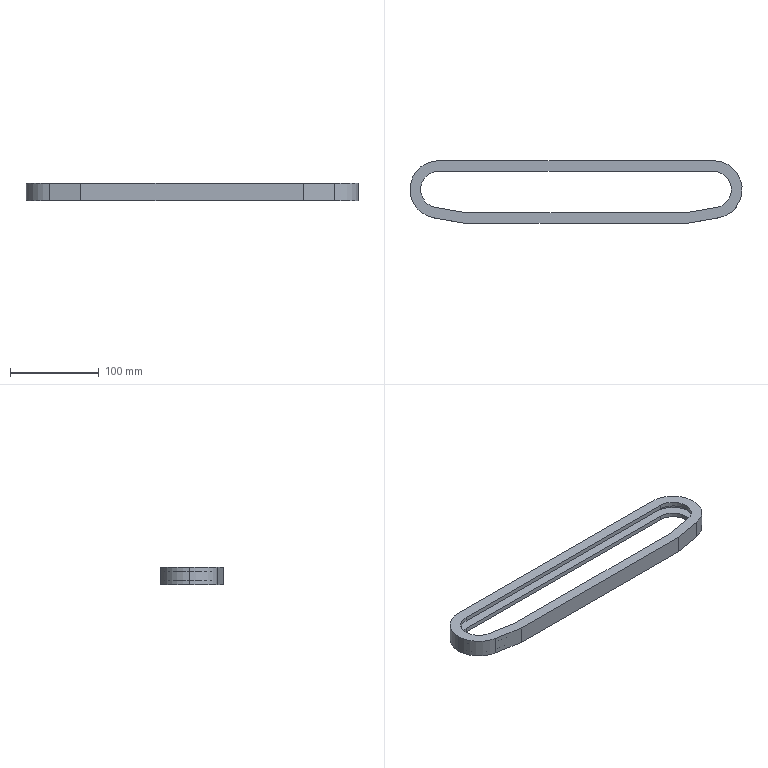Part | SolidWorks | features Extrusion 1, ICE 1 | 1 solid | 32 faces | box 375 x 70.699 x 20 mm | volume 102724 mm3 | plane 20 | cylinder 12 | commonest cylinder face diameters 41 x6 63 x3 65 x3
STEP:
#1=CARTESIAN_POINT('',(186.5,0.,-5.));
#2=VERTEX_POINT('',#1);
#3=CARTESIAN_POINT('',(155.,31.5,-5.));
#4=VERTEX_POINT('',#3);
#5=CARTESIAN_POINT('',(155.,0.,-5.));
#6=DIRECTION('',(0.,0.,1.));
#7=DIRECTION('',(1.,0.,0.));
#8=AXIS2_PLACEMENT_3D('',#5,#6,#7);
#9=CIRCLE('',#8,31.5);
#10=EDGE_CURVE('',#2,#4,#9,.T.);
#11=ORIENTED_EDGE('',*,*,#10,.F.);
#12=CARTESIAN_POINT('',(186.5,0.,5.));
#13=VERTEX_POINT('',#12);
#14=CARTESIAN_POINT('',(186.5,0.,-5.));
#15=DIRECTION('',(0.,0.,1.));
#16=VECTOR('',#15,1000.);
#17=LINE('',#14,#16);
#18=EDGE_CURVE('',#2,#13,#17,.T.);
#19=ORIENTED_EDGE('',*,*,#18,.T.);
#20=CARTESIAN_POINT('',(155.,31.5,5.));
#21=VERTEX_POINT('',#20);
#22=CARTESIAN_POINT('',(155.,0.,5.));
#23=DIRECTION('',(0.,0.,1.));
#24=DIRECTION('',(1.,0.,0.));
#25=AXIS2_PLACEMENT_3D('',#22,#23,#24);
#26=CIRCLE('',#25,31.5);
#27=EDGE_CURVE('',#13,#21,#26,.T.);
#28=ORIENTED_EDGE('',*,*,#27,.T.);
#29=CARTESIAN_POINT('',(155.,31.5,-5.));
#30=DIRECTION('',(0.,0.,1.));
#31=VECTOR('',#30,1000.);
#32=LINE('',#29,#31);
#33=EDGE_CURVE('',#4,#21,#32,.T.);
#34=ORIENTED_EDGE('',*,*,#33,.F.);
#35=EDGE_LOOP('',(#11,#19,#28,#34));
#36=FACE_OUTER_BOUND('',#35,.T.);
#37=CARTESIAN_POINT('',(155.,0.,-5.));
#38=DIRECTION('',(0.,0.,1.));
#39=DIRECTION('',(1.,0.,0.));
#40=AXIS2_PLACEMENT_3D('',#37,#38,#39);
#41=CYLINDRICAL_SURFACE('',#40,31.5);
#42=ADVANCED_FACE('',(#36),#41,.F.);
#43=CARTESIAN_POINT('',(-155.,20.5,10.));
#44=VERTEX_POINT('',#43);
#45=CARTESIAN_POINT('',(-175.5,0.,10.));
#46=VERTEX_POINT('',#45);
#47=CARTESIAN_POINT('',(-155.,0.,10.));
#48=DIRECTION('',(0.,0.,1.));
#49=DIRECTION('',(1.,0.,0.));
#50=AXIS2_PLACEMENT_3D('',#47,#48,#49);
#51=CIRCLE('',#50,20.5);
#52=EDGE_CURVE('',#44,#46,#51,.T.);
#53=ORIENTED_EDGE('',*,*,#52,.T.);
#54=CARTESIAN_POINT('',(-175.5,0.,5.));
#55=VERTEX_POINT('',#54);
#56=CARTESIAN_POINT('',(-175.5,0.,10.));
#57=DIRECTION('',(0.,0.,-1.));
#58=VECTOR('',#57,1000.);
#59=LINE('',#56,#58);
#60=EDGE_CURVE('',#46,#55,#59,.T.);
#61=ORIENTED_EDGE('',*,*,#60,.T.);
#62=CARTESIAN_POINT('',(-155.,20.5,5.));
#63=VERTEX_POINT('',#62);
#64=CARTESIAN_POINT('',(-155.,0.,5.));
#65=DIRECTION('',(0.,0.,1.));
#66=DIRECTION('',(1.,0.,0.));
#67=AXIS2_PLACEMENT_3D('',#64,#65,#66);
#68=CIRCLE('',#67,20.5);
#69=EDGE_CURVE('',#63,#55,#68,.T.);
#70=ORIENTED_EDGE('',*,*,#69,.F.);
#71=CARTESIAN_POINT('',(-155.,20.5,10.));
#72=DIRECTION('',(0.,0.,-1.));
#73=VECTOR('',#72,1000.);
#74=LINE('',#71,#73);
#75=EDGE_CURVE('',#44,#63,#74,.T.);
#76=ORIENTED_EDGE('',*,*,#75,.F.);
#77=EDGE_LOOP('',(#53,#61,#70,#76));
#78=FACE_OUTER_BOUND('',#77,.T.);
#79=CARTESIAN_POINT('',(-155.,0.,10.));
#80=DIRECTION('',(0.,0.,-1.));
#81=DIRECTION('',(-1.,0.,0.));
#82=AXIS2_PLACEMENT_3D('',#79,#80,#81);
#83=CYLINDRICAL_SURFACE('',#82,20.5);
#84=ADVANCED_FACE('',(#78),#83,.F.);
#85=CARTESIAN_POINT('',(-187.5,0.,10.));
#86=VERTEX_POINT('',#85);
#87=CARTESIAN_POINT('',(-160.644,-32.006,10.));
#88=VERTEX_POINT('',#87);
#89=CARTESIAN_POINT('',(-155.,0.,10.));
#90=DIRECTION('',(0.,0.,1.));
#91=DIRECTION('',(1.,0.,0.));
#92=AXIS2_PLACEMENT_3D('',#89,#90,#91);
#93=CIRCLE('',#92,32.5);
#94=EDGE_CURVE('',#86,#88,#93,.T.);
#95=ORIENTED_EDGE('',*,*,#94,.F.);
#96=CARTESIAN_POINT('',(-187.5,0.,-10.));
#97=VERTEX_POINT('',#96);
#98=CARTESIAN_POINT('',(-187.5,0.,10.));
#99=DIRECTION('',(0.,0.,-1.));
#100=VECTOR('',#99,1000.);
#101=LINE('',#98,#100);
#102=EDGE_CURVE('',#86,#97,#101,.T.);
#103=ORIENTED_EDGE('',*,*,#102,.T.);
#104=CARTESIAN_POINT('',(-160.644,-32.006,-10.));
#105=VERTEX_POINT('',#104);
#106=CARTESIAN_POINT('',(-155.,0.,-10.));
#107=DIRECTION('',(0.,0.,1.));
#108=DIRECTION('',(1.,0.,0.));
#109=AXIS2_PLACEMENT_3D('',#106,#107,#108);
#110=CIRCLE('',#109,32.5);
#111=EDGE_CURVE('',#97,#105,#110,.T.);
#112=ORIENTED_EDGE('',*,*,#111,.T.);
#113=CARTESIAN_POINT('',(-160.644,-32.006,10.));
#114=DIRECTION('',(0.,0.,-1.));
#115=VECTOR('',#114,1000.);
#116=LINE('',#113,#115);
#117=EDGE_CURVE('',#88,#105,#116,.T.);
#118=ORIENTED_EDGE('',*,*,#117,.F.);
#119=EDGE_LOOP('',(#95,#103,#112,#118));
#120=FACE_OUTER_BOUND('',#119,.T.);
#121=CARTESIAN_POINT('',(-155.,0.,10.));
#122=DIRECTION('',(0.,0.,-1.));
#123=DIRECTION('',(-1.,0.,0.));
#124=AXIS2_PLACEMENT_3D('',#121,#122,#123);
#125=CYLINDRICAL_SURFACE('',#124,32.5);
#126=ADVANCED_FACE('',(#120),#125,.T.);
#127=CARTESIAN_POINT('',(-155.,20.5,-5.));
#128=VERTEX_POINT('',#127);
#129=CARTESIAN_POINT('',(-175.5,0.,-5.));
#130=VERTEX_POINT('',#129);
#131=CARTESIAN_POINT('',(-155.,0.,-5.));
#132=DIRECTION('',(0.,0.,1.));
#133=DIRECTION('',(1.,0.,0.));
#134=AXIS2_PLACEMENT_3D('',#131,#132,#133);
#135=CIRCLE('',#134,20.5);
#136=EDGE_CURVE('',#128,#130,#135,.T.);
#137=ORIENTED_EDGE('',*,*,#136,.T.);
#138=CARTESIAN_POINT('',(-175.5,0.,-10.));
#139=VERTEX_POINT('',#138);
#140=CARTESIAN_POINT('',(-175.5,0.,10.));
#141=DIRECTION('',(0.,0.,-1.));
#142=VECTOR('',#141,1000.);
#143=LINE('',#140,#142);
#144=EDGE_CURVE('',#130,#139,#143,.T.);
#145=ORIENTED_EDGE('',*,*,#144,.T.);
#146=CARTESIAN_POINT('',(-155.,20.5,-10.));
#147=VERTEX_POINT('',#146);
#148=CARTESIAN_POINT('',(-155.,0.,-10.));
#149=DIRECTION('',(0.,0.,1.));
#150=DIRECTION('',(1.,0.,0.));
#151=AXIS2_PLACEMENT_3D('',#148,#149,#150);
#152=CIRCLE('',#151,20.5);
#153=EDGE_CURVE('',#147,#139,#152,.T.);
#154=ORIENTED_EDGE('',*,*,#153,.F.);
#155=CARTESIAN_POINT('',(-155.,20.5,10.));
#156=DIRECTION('',(0.,0.,-1.));
#157=VECTOR('',#156,1000.);
#158=LINE('',#155,#157);
#159=EDGE_CURVE('',#128,#147,#158,.T.);
#160=ORIENTED_EDGE('',*,*,#159,.F.);
#161=EDGE_LOOP('',(#137,#145,#154,#160));
#162=FACE_OUTER_BOUND('',#161,.T.);
#163=CARTESIAN_POINT('',(-155.,0.,10.));
#164=DIRECTION('',(0.,0.,-1.));
#165=DIRECTION('',(-1.,0.,0.));
#166=AXIS2_PLACEMENT_3D('',#163,#164,#165);
#167=CYLINDRICAL_SURFACE('',#166,20.5);
#168=ADVANCED_FACE('',(#162),#167,.F.);
#169=ORIENTED_EDGE('',*,*,#144,.F.);
#170=CARTESIAN_POINT('',(-158.56,-20.189,-5.));
#171=VERTEX_POINT('',#170);
#172=CARTESIAN_POINT('',(-155.,0.,-5.));
#173=DIRECTION('',(0.,0.,1.));
#174=DIRECTION('',(1.,0.,0.));
#175=AXIS2_PLACEMENT_3D('',#172,#173,#174);
#176=CIRCLE('',#175,20.5);
#177=EDGE_CURVE('',#130,#171,#176,.T.);
#178=ORIENTED_EDGE('',*,*,#177,.T.);
#179=CARTESIAN_POINT('',(-158.56,-20.189,-10.));
#180=VERTEX_POINT('',#179);
#181=CARTESIAN_POINT('',(-158.56,-20.189,10.));
#182=DIRECTION('',(0.,0.,-1.));
#183=VECTOR('',#182,1000.);
#184=LINE('',#181,#183);
#185=EDGE_CURVE('',#171,#180,#184,.T.);
#186=ORIENTED_EDGE('',*,*,#185,.T.);
#187=CARTESIAN_POINT('',(-155.,0.,-10.));
#188=DIRECTION('',(0.,0.,1.));
#189=DIRECTION('',(1.,0.,0.));
#190=AXIS2_PLACEMENT_3D('',#187,#188,#189);
#191=CIRCLE('',#190,20.5);
#192=EDGE_CURVE('',#139,#180,#191,.T.);
#193=ORIENTED_EDGE('',*,*,#192,.F.);
#194=EDGE_LOOP('',(#169,#178,#186,#193));
#195=FACE_OUTER_BOUND('',#194,.T.);
#196=CARTESIAN_POINT('',(-155.,0.,10.));
#197=DIRECTION('',(0.,0.,-1.));
#198=DIRECTION('',(-1.,0.,0.));
#199=AXIS2_PLACEMENT_3D('',#196,#197,#198);
#200=CYLINDRICAL_SURFACE('',#199,20.5);
#201=ADVANCED_FACE('',(#195),#200,.F.);
#202=ORIENTED_EDGE('',*,*,#185,.F.);
#203=CARTESIAN_POINT('',(-124.475,-26.199,-5.));
#204=VERTEX_POINT('',#203);
#205=CARTESIAN_POINT('',(-124.475,-26.199,-5.));
#206=DIRECTION('',(0.9848,-0.1736,0.));
#207=VECTOR('',#206,1000.);
#208=LINE('',#205,#207);
#209=EDGE_CURVE('',#171,#204,#208,.T.);
#210=ORIENTED_EDGE('',*,*,#209,.T.);
#211=CARTESIAN_POINT('',(-124.475,-26.199,-10.));
#212=VERTEX_POINT('',#211);
#213=CARTESIAN_POINT('',(-124.475,-26.199,10.));
#214=DIRECTION('',(0.,0.,-1.));
#215=VECTOR('',#214,1000.);
#216=LINE('',#213,#215);
#217=EDGE_CURVE('',#204,#212,#216,.T.);
#218=ORIENTED_EDGE('',*,*,#217,.T.);
#219=CARTESIAN_POINT('',(-124.475,-26.199,-10.));
#220=DIRECTION('',(0.9848,-0.1736,0.));
#221=VECTOR('',#220,1000.);
#222=LINE('',#219,#221);
#223=EDGE_CURVE('',#180,#212,#222,.T.);
#224=ORIENTED_EDGE('',*,*,#223,.F.);
#225=EDGE_LOOP('',(#202,#210,#218,#224));
#226=FACE_OUTER_BOUND('',#225,.T.);
#227=CARTESIAN_POINT('',(-124.475,-26.199,10.));
#228=DIRECTION('',(0.1736,0.9848,0.));
#229=DIRECTION('',(-0.9848,0.1736,0.));
#230=AXIS2_PLACEMENT_3D('',#227,#228,#229);
#231=PLANE('',#230);
#232=ADVANCED_FACE('',(#226),#231,.T.);
#233=ORIENTED_EDGE('',*,*,#217,.F.);
#234=CARTESIAN_POINT('',(124.475,-26.199,-5.));
#235=VERTEX_POINT('',#234);
#236=CARTESIAN_POINT('',(-124.475,-26.199,-5.));
#237=DIRECTION('',(1.,0.,0.));
#238=VECTOR('',#237,1000.);
#239=LINE('',#236,#238);
#240=EDGE_CURVE('',#204,#235,#239,.T.);
#241=ORIENTED_EDGE('',*,*,#240,.T.);
#242=CARTESIAN_POINT('',(124.475,-26.199,-10.));
#243=VERTEX_POINT('',#242);
#244=CARTESIAN_POINT('',(124.475,-26.199,10.));
#245=DIRECTION('',(0.,0.,-1.));
#246=VECTOR('',#245,1000.);
#247=LINE('',#244,#246);
#248=EDGE_CURVE('',#235,#243,#247,.T.);
#249=ORIENTED_EDGE('',*,*,#248,.T.);
#250=CARTESIAN_POINT('',(-124.475,-26.199,-10.));
#251=DIRECTION('',(1.,0.,0.));
#252=VECTOR('',#251,1000.);
#253=LINE('',#250,#252);
#254=EDGE_CURVE('',#212,#243,#253,.T.);
#255=ORIENTED_EDGE('',*,*,#254,.F.);
#256=EDGE_LOOP('',(#233,#241,#249,#255));
#257=FACE_OUTER_BOUND('',#256,.T.);
#258=CARTESIAN_POINT('',(-124.475,-26.199,10.));
#259=DIRECTION('',(0.,1.,0.));
#260=DIRECTION('',(0.,0.,1.));
#261=AXIS2_PLACEMENT_3D('',#258,#259,#260);
#262=PLANE('',#261);
#263=ADVANCED_FACE('',(#257),#262,.T.);
#264=ORIENTED_EDGE('',*,*,#248,.F.);
#265=CARTESIAN_POINT('',(158.56,-20.189,-5.));
#266=VERTEX_POINT('',#265);
#267=CARTESIAN_POINT('',(124.475,-26.199,-5.));
#268=DIRECTION('',(0.9848,0.1736,0.));
#269=VECTOR('',#268,1000.);
#270=LINE('',#267,#269);
#271=EDGE_CURVE('',#235,#266,#270,.T.);
#272=ORIENTED_EDGE('',*,*,#271,.T.);
#273=CARTESIAN_POINT('',(158.56,-20.189,-10.));
#274=VERTEX_POINT('',#273);
#275=CARTESIAN_POINT('',(158.56,-20.189,10.));
#276=DIRECTION('',(0.,0.,-1.));
#277=VECTOR('',#276,1000.);
#278=LINE('',#275,#277);
#279=EDGE_CURVE('',#266,#274,#278,.T.);
#280=ORIENTED_EDGE('',*,*,#279,.T.);
#281=CARTESIAN_POINT('',(124.475,-26.199,-10.));
#282=DIRECTION('',(0.9848,0.1736,0.));
#283=VECTOR('',#282,1000.);
#284=LINE('',#281,#283);
#285=EDGE_CURVE('',#243,#274,#284,.T.);
#286=ORIENTED_EDGE('',*,*,#285,.F.);
#287=EDGE_LOOP('',(#264,#272,#280,#286));
#288=FACE_OUTER_BOUND('',#287,.T.);
#289=CARTESIAN_POINT('',(124.475,-26.199,10.));
#290=DIRECTION('',(-0.1736,0.9848,0.));
#291=DIRECTION('',(-0.9848,-0.1736,0.));
#292=AXIS2_PLACEMENT_3D('',#289,#290,#291);
#293=PLANE('',#292);
#294=ADVANCED_FACE('',(#288),#293,.T.);
#295=ORIENTED_EDGE('',*,*,#279,.F.);
#296=CARTESIAN_POINT('',(155.,20.5,-5.));
#297=VERTEX_POINT('',#296);
#298=CARTESIAN_POINT('',(155.,0.,-5.));
#299=DIRECTION('',(0.,0.,1.));
#300=DIRECTION('',(1.,0.,0.));
#301=AXIS2_PLACEMENT_3D('',#298,#299,#300);
#302=CIRCLE('',#301,20.5);
#303=EDGE_CURVE('',#266,#297,#302,.T.);
#304=ORIENTED_EDGE('',*,*,#303,.T.);
#305=CARTESIAN_POINT('',(155.,20.5,-10.));
#306=VERTEX_POINT('',#305);
#307=CARTESIAN_POINT('',(155.,20.5,10.));
#308=DIRECTION('',(0.,0.,-1.));
#309=VECTOR('',#308,1000.);
#310=LINE('',#307,#309);
#311=EDGE_CURVE('',#297,#306,#310,.T.);
#312=ORIENTED_EDGE('',*,*,#311,.T.);
#313=CARTESIAN_POINT('',(155.,0.,-10.));
#314=DIRECTION('',(0.,0.,1.));
#315=DIRECTION('',(-1.,0.,0.));
#316=AXIS2_PLACEMENT_3D('',#313,#314,#315);
#317=CIRCLE('',#316,20.5);
#318=EDGE_CURVE('',#274,#306,#317,.T.);
#319=ORIENTED_EDGE('',*,*,#318,.F.);
#320=EDGE_LOOP('',(#295,#304,#312,#319));
#321=FACE_OUTER_BOUND('',#320,.T.);
#322=CARTESIAN_POINT('',(155.,0.,10.));
#323=DIRECTION('',(0.,0.,-1.));
#324=DIRECTION('',(-1.,0.,0.));
#325=AXIS2_PLACEMENT_3D('',#322,#323,#324);
#326=CYLINDRICAL_SURFACE('',#325,20.5);
#327=ADVANCED_FACE('',(#321),#326,.F.);
#328=ORIENTED_EDGE('',*,*,#311,.F.);
#329=CARTESIAN_POINT('',(-155.,20.5,-5.));
#330=DIRECTION('',(-1.,0.,0.));
#331=VECTOR('',#330,1000.);
#332=LINE('',#329,#331);
#333=EDGE_CURVE('',#297,#128,#332,.T.);
#334=ORIENTED_EDGE('',*,*,#333,.T.);
#335=ORIENTED_EDGE('',*,*,#159,.T.);
#336=CARTESIAN_POINT('',(-155.,20.5,-10.));
#337=DIRECTION('',(-1.,0.,0.));
#338=VECTOR('',#337,1000.);
#339=LINE('',#336,#338);
#340=EDGE_CURVE('',#306,#147,#339,.T.);
#341=ORIENTED_EDGE('',*,*,#340,.F.);
#342=EDGE_LOOP('',(#328,#334,#335,#341));
#343=FACE_OUTER_BOUND('',#342,.T.);
#344=CARTESIAN_POINT('',(-155.,20.5,10.));
#345=DIRECTION('',(0.,-1.,0.));
#346=DIRECTION('',(0.,0.,-1.));
#347=AXIS2_PLACEMENT_3D('',#344,#345,#346);
#348=PLANE('',#347);
#349=ADVANCED_FACE('',(#343),#348,.T.);
#350=CARTESIAN_POINT('',(-155.,32.5,10.));
#351=VERTEX_POINT('',#350);
#352=CARTESIAN_POINT('',(-155.,0.,10.));
#353=DIRECTION('',(0.,0.,1.));
#354=DIRECTION('',(1.,0.,0.));
#355=AXIS2_PLACEMENT_3D('',#352,#353,#354);
#356=CIRCLE('',#355,32.5);
#357=EDGE_CURVE('',#351,#86,#356,.T.);
#358=ORIENTED_EDGE('',*,*,#357,.T.);
#359=ORIENTED_EDGE('',*,*,#94,.T.);
#360=CARTESIAN_POINT('',(-125.525,-38.199,10.));
#361=VERTEX_POINT('',#360);
#362=CARTESIAN_POINT('',(-125.525,-38.199,10.));
#363=DIRECTION('',(0.9848,-0.1736,0.));
#364=VECTOR('',#363,1000.);
#365=LINE('',#362,#364);
#366=EDGE_CURVE('',#88,#361,#365,.T.);
#367=ORIENTED_EDGE('',*,*,#366,.T.);
#368=CARTESIAN_POINT('',(125.525,-38.199,10.));
#369=VERTEX_POINT('',#368);
#370=CARTESIAN_POINT('',(-125.525,-38.199,10.));
#371=DIRECTION('',(1.,0.,0.));
#372=VECTOR('',#371,1000.);
#373=LINE('',#370,#372);
#374=EDGE_CURVE('',#361,#369,#373,.T.);
#375=ORIENTED_EDGE('',*,*,#374,.T.);
#376=CARTESIAN_POINT('',(160.644,-32.006,10.));
#377=VERTEX_POINT('',#376);
#378=CARTESIAN_POINT('',(125.525,-38.199,10.));
#379=DIRECTION('',(0.9848,0.1736,0.));
#380=VECTOR('',#379,1000.);
#381=LINE('',#378,#380);
#382=EDGE_CURVE('',#369,#377,#381,.T.);
#383=ORIENTED_EDGE('',*,*,#382,.T.);
#384=CARTESIAN_POINT('',(155.,32.5,10.));
#385=VERTEX_POINT('',#384);
#386=CARTESIAN_POINT('',(155.,0.,10.));
#387=DIRECTION('',(0.,0.,1.));
#388=DIRECTION('',(-1.,0.,0.));
#389=AXIS2_PLACEMENT_3D('',#386,#387,#388);
#390=CIRCLE('',#389,32.5);
#391=EDGE_CURVE('',#377,#385,#390,.T.);
#392=ORIENTED_EDGE('',*,*,#391,.T.);
#393=CARTESIAN_POINT('',(-155.,32.5,10.));
#394=DIRECTION('',(-1.,0.,0.));
#395=VECTOR('',#394,1000.);
#396=LINE('',#393,#395);
#397=EDGE_CURVE('',#385,#351,#396,.T.);
#398=ORIENTED_EDGE('',*,*,#397,.T.);
#399=EDGE_LOOP('',(#358,#359,#367,#375,#383,#392,#398));
#400=FACE_OUTER_BOUND('',#399,.T.);
#401=CARTESIAN_POINT('',(-158.56,-20.189,10.));
#402=VERTEX_POINT('',#401);
#403=CARTESIAN_POINT('',(-124.475,-26.199,10.));
#404=VERTEX_POINT('',#403);
#405=CARTESIAN_POINT('',(-124.475,-26.199,10.));
#406=DIRECTION('',(0.9848,-0.1736,0.));
#407=VECTOR('',#406,1000.);
#408=LINE('',#405,#407);
#409=EDGE_CURVE('',#402,#404,#408,.T.);
#410=ORIENTED_EDGE('',*,*,#409,.F.);
#411=CARTESIAN_POINT('',(-155.,0.,10.));
#412=DIRECTION('',(0.,0.,1.));
#413=DIRECTION('',(1.,0.,0.));
#414=AXIS2_PLACEMENT_3D('',#411,#412,#413);
#415=CIRCLE('',#414,20.5);
#416=EDGE_CURVE('',#46,#402,#415,.T.);
#417=ORIENTED_EDGE('',*,*,#416,.F.);
#418=ORIENTED_EDGE('',*,*,#52,.F.);
#419=CARTESIAN_POINT('',(155.,20.5,10.));
#420=VERTEX_POINT('',#419);
#421=CARTESIAN_POINT('',(-155.,20.5,10.));
#422=DIRECTION('',(-1.,0.,0.));
#423=VECTOR('',#422,1000.);
#424=LINE('',#421,#423);
#425=EDGE_CURVE('',#420,#44,#424,.T.);
#426=ORIENTED_EDGE('',*,*,#425,.F.);
#427=CARTESIAN_POINT('',(158.56,-20.189,10.));
#428=VERTEX_POINT('',#427);
#429=CARTESIAN_POINT('',(155.,0.,10.));
#430=DIRECTION('',(0.,0.,1.));
#431=DIRECTION('',(-1.,0.,0.));
#432=AXIS2_PLACEMENT_3D('',#429,#430,#431);
#433=CIRCLE('',#432,20.5);
#434=EDGE_CURVE('',#428,#420,#433,.T.);
#435=ORIENTED_EDGE('',*,*,#434,.F.);
#436=CARTESIAN_POINT('',(124.475,-26.199,10.));
#437=VERTEX_POINT('',#436);
#438=CARTESIAN_POINT('',(124.475,-26.199,10.));
#439=DIRECTION('',(0.9848,0.1736,0.));
#440=VECTOR('',#439,1000.);
#441=LINE('',#438,#440);
#442=EDGE_CURVE('',#437,#428,#441,.T.);
#443=ORIENTED_EDGE('',*,*,#442,.F.);
#444=CARTESIAN_POINT('',(-124.475,-26.199,10.));
#445=DIRECTION('',(1.,0.,0.));
#446=VECTOR('',#445,1000.);
#447=LINE('',#444,#446);
#448=EDGE_CURVE('',#404,#437,#447,.T.);
#449=ORIENTED_EDGE('',*,*,#448,.F.);
#450=EDGE_LOOP('',(#410,#417,#418,#426,#435,#443,#449));
#451=FACE_BOUND('',#450,.T.);
#452=CARTESIAN_POINT('',(-155.,0.,10.));
#453=DIRECTION('',(0.,0.,1.));
#454=DIRECTION('',(1.,0.,0.));
#455=AXIS2_PLACEMENT_3D('',#452,#453,#454);
#456=PLANE('',#455);
#457=ADVANCED_FACE('',(#400,#451),#456,.T.);
#458=CARTESIAN_POINT('',(-155.,32.5,-10.));
#459=VERTEX_POINT('',#458);
#460=CARTESIAN_POINT('',(-155.,0.,-10.));
#461=DIRECTION('',(0.,0.,1.));
#462=DIRECTION('',(1.,0.,0.));
#463=AXIS2_PLACEMENT_3D('',#460,#461,#462);
#464=CIRCLE('',#463,32.5);
#465=EDGE_CURVE('',#459,#97,#464,.T.);
#466=ORIENTED_EDGE('',*,*,#465,.F.);
#467=CARTESIAN_POINT('',(155.,32.5,-10.));
#468=VERTEX_POINT('',#467);
#469=CARTESIAN_POINT('',(-155.,32.5,-10.));
#470=DIRECTION('',(-1.,0.,0.));
#471=VECTOR('',#470,1000.);
#472=LINE('',#469,#471);
#473=EDGE_CURVE('',#468,#459,#472,.T.);
#474=ORIENTED_EDGE('',*,*,#473,.F.);
#475=CARTESIAN_POINT('',(160.644,-32.006,-10.));
#476=VERTEX_POINT('',#475);
#477=CARTESIAN_POINT('',(155.,0.,-10.));
#478=DIRECTION('',(0.,0.,1.));
#479=DIRECTION('',(-1.,0.,0.));
#480=AXIS2_PLACEMENT_3D('',#477,#478,#479);
#481=CIRCLE('',#480,32.5);
#482=EDGE_CURVE('',#476,#468,#481,.T.);
#483=ORIENTED_EDGE('',*,*,#482,.F.);
#484=CARTESIAN_POINT('',(125.525,-38.199,-10.));
#485=VERTEX_POINT('',#484);
#486=CARTESIAN_POINT('',(125.525,-38.199,-10.));
#487=DIRECTION('',(0.9848,0.1736,0.));
#488=VECTOR('',#487,1000.);
#489=LINE('',#486,#488);
#490=EDGE_CURVE('',#485,#476,#489,.T.);
#491=ORIENTED_EDGE('',*,*,#490,.F.);
#492=CARTESIAN_POINT('',(-125.525,-38.199,-10.));
#493=VERTEX_POINT('',#492);
#494=CARTESIAN_POINT('',(-125.525,-38.199,-10.));
#495=DIRECTION('',(1.,0.,0.));
#496=VECTOR('',#495,1000.);
#497=LINE('',#494,#496);
#498=EDGE_CURVE('',#493,#485,#497,.T.);
#499=ORIENTED_EDGE('',*,*,#498,.F.);
#500=CARTESIAN_POINT('',(-125.525,-38.199,-10.));
#501=DIRECTION('',(0.9848,-0.1736,0.));
#502=VECTOR('',#501,1000.);
#503=LINE('',#500,#502);
#504=EDGE_CURVE('',#105,#493,#503,.T.);
#505=ORIENTED_EDGE('',*,*,#504,.F.);
#506=ORIENTED_EDGE('',*,*,#111,.F.);
#507=EDGE_LOOP('',(#466,#474,#483,#491,#499,#505,#506));
#508=FACE_OUTER_BOUND('',#507,.T.);
#509=ORIENTED_EDGE('',*,*,#153,.T.);
#510=ORIENTED_EDGE('',*,*,#192,.T.);
#511=ORIENTED_EDGE('',*,*,#223,.T.);
#512=ORIENTED_EDGE('',*,*,#254,.T.);
#513=ORIENTED_EDGE('',*,*,#285,.T.);
#514=ORIENTED_EDGE('',*,*,#318,.T.);
#515=ORIENTED_EDGE('',*,*,#340,.T.);
#516=EDGE_LOOP('',(#509,#510,#511,#512,#513,#514,#515));
#517=FACE_BOUND('',#516,.T.);
#518=CARTESIAN_POINT('',(-155.,0.,-10.));
#519=DIRECTION('',(0.,0.,1.));
#520=DIRECTION('',(1.,0.,0.));
#521=AXIS2_PLACEMENT_3D('',#518,#519,#520);
#522=PLANE('',#521);
#523=ADVANCED_FACE('',(#508,#517),#522,.F.);
#524=ORIENTED_EDGE('',*,*,#102,.F.);
#525=ORIENTED_EDGE('',*,*,#357,.F.);
#526=CARTESIAN_POINT('',(-155.,32.5,10.));
#527=DIRECTION('',(0.,0.,-1.));
#528=VECTOR('',#527,1000.);
#529=LINE('',#526,#528);
#530=EDGE_CURVE('',#351,#459,#529,.T.);
#531=ORIENTED_EDGE('',*,*,#530,.T.);
#532=ORIENTED_EDGE('',*,*,#465,.T.);
#533=EDGE_LOOP('',(#524,#525,#531,#532));
#534=FACE_OUTER_BOUND('',#533,.T.);
#535=CARTESIAN_POINT('',(-155.,0.,10.));
#536=DIRECTION('',(0.,0.,-1.));
#537=DIRECTION('',(-1.,0.,0.));
#538=AXIS2_PLACEMENT_3D('',#535,#536,#537);
#539=CYLINDRICAL_SURFACE('',#538,32.5);
#540=ADVANCED_FACE('',(#534),#539,.T.);
#541=ORIENTED_EDGE('',*,*,#504,.T.);
#542=CARTESIAN_POINT('',(-125.525,-38.199,10.));
#543=DIRECTION('',(0.,0.,-1.));
#544=VECTOR('',#543,1000.);
#545=LINE('',#542,#544);
#546=EDGE_CURVE('',#361,#493,#545,.T.);
#547=ORIENTED_EDGE('',*,*,#546,.F.);
#548=ORIENTED_EDGE('',*,*,#366,.F.);
#549=ORIENTED_EDGE('',*,*,#117,.T.);
#550=EDGE_LOOP('',(#541,#547,#548,#549));
#551=FACE_OUTER_BOUND('',#550,.T.);
#552=CARTESIAN_POINT('',(-125.525,-38.199,10.));
#553=DIRECTION('',(0.1736,0.9848,0.));
#554=DIRECTION('',(-0.9848,0.1736,0.));
#555=AXIS2_PLACEMENT_3D('',#552,#553,#554);
#556=PLANE('',#555);
#557=ADVANCED_FACE('',(#551),#556,.F.);
#558=ORIENTED_EDGE('',*,*,#498,.T.);
#559=CARTESIAN_POINT('',(125.525,-38.199,10.));
#560=DIRECTION('',(0.,0.,-1.));
#561=VECTOR('',#560,1000.);
#562=LINE('',#559,#561);
#563=EDGE_CURVE('',#369,#485,#562,.T.);
#564=ORIENTED_EDGE('',*,*,#563,.F.);
#565=ORIENTED_EDGE('',*,*,#374,.F.);
#566=ORIENTED_EDGE('',*,*,#546,.T.);
#567=EDGE_LOOP('',(#558,#564,#565,#566));
#568=FACE_OUTER_BOUND('',#567,.T.);
#569=CARTESIAN_POINT('',(-125.525,-38.199,10.));
#570=DIRECTION('',(0.,1.,0.));
#571=DIRECTION('',(0.,0.,1.));
#572=AXIS2_PLACEMENT_3D('',#569,#570,#571);
#573=PLANE('',#572);
#574=ADVANCED_FACE('',(#568),#573,.F.);
#575=ORIENTED_EDGE('',*,*,#490,.T.);
#576=CARTESIAN_POINT('',(160.644,-32.006,10.));
#577=DIRECTION('',(0.,0.,-1.));
#578=VECTOR('',#577,1000.);
#579=LINE('',#576,#578);
#580=EDGE_CURVE('',#377,#476,#579,.T.);
#581=ORIENTED_EDGE('',*,*,#580,.F.);
#582=ORIENTED_EDGE('',*,*,#382,.F.);
#583=ORIENTED_EDGE('',*,*,#563,.T.);
#584=EDGE_LOOP('',(#575,#581,#582,#583));
#585=FACE_OUTER_BOUND('',#584,.T.);
#586=CARTESIAN_POINT('',(125.525,-38.199,10.));
#587=DIRECTION('',(-0.1736,0.9848,0.));
#588=DIRECTION('',(-0.9848,-0.1736,0.));
#589=AXIS2_PLACEMENT_3D('',#586,#587,#588);
#590=PLANE('',#589);
#591=ADVANCED_FACE('',(#585),#590,.F.);
#592=ORIENTED_EDGE('',*,*,#482,.T.);
#593=CARTESIAN_POINT('',(155.,32.5,10.));
#594=DIRECTION('',(0.,0.,-1.));
#595=VECTOR('',#594,1000.);
#596=LINE('',#593,#595);
#597=EDGE_CURVE('',#385,#468,#596,.T.);
#598=ORIENTED_EDGE('',*,*,#597,.F.);
#599=ORIENTED_EDGE('',*,*,#391,.F.);
#600=ORIENTED_EDGE('',*,*,#580,.T.);
#601=EDGE_LOOP('',(#592,#598,#599,#600));
#602=FACE_OUTER_BOUND('',#601,.T.);
#603=CARTESIAN_POINT('',(155.,0.,10.));
#604=DIRECTION('',(0.,0.,-1.));
#605=DIRECTION('',(-1.,0.,0.));
#606=AXIS2_PLACEMENT_3D('',#603,#604,#605);
#607=CYLINDRICAL_SURFACE('',#606,32.5);
#608=ADVANCED_FACE('',(#602),#607,.T.);
#609=ORIENTED_EDGE('',*,*,#473,.T.);
#610=ORIENTED_EDGE('',*,*,#530,.F.);
#611=ORIENTED_EDGE('',*,*,#397,.F.);
#612=ORIENTED_EDGE('',*,*,#597,.T.);
#613=EDGE_LOOP('',(#609,#610,#611,#612));
#614=FACE_OUTER_BOUND('',#613,.T.);
#615=CARTESIAN_POINT('',(-155.,32.5,10.));
#616=DIRECTION('',(0.,-1.,0.));
#617=DIRECTION('',(0.,0.,-1.));
#618=AXIS2_PLACEMENT_3D('',#615,#616,#617);
#619=PLANE('',#618);
#620=ADVANCED_FACE('',(#614),#619,.F.);
#621=ORIENTED_EDGE('',*,*,#60,.F.);
#622=ORIENTED_EDGE('',*,*,#416,.T.);
#623=CARTESIAN_POINT('',(-158.56,-20.189,5.));
#624=VERTEX_POINT('',#623);
#625=CARTESIAN_POINT('',(-158.56,-20.189,10.));
#626=DIRECTION('',(0.,0.,-1.));
#627=VECTOR('',#626,1000.);
#628=LINE('',#625,#627);
#629=EDGE_CURVE('',#402,#624,#628,.T.);
#630=ORIENTED_EDGE('',*,*,#629,.T.);
#631=CARTESIAN_POINT('',(-155.,0.,5.));
#632=DIRECTION('',(0.,0.,1.));
#633=DIRECTION('',(1.,0.,0.));
#634=AXIS2_PLACEMENT_3D('',#631,#632,#633);
#635=CIRCLE('',#634,20.5);
#636=EDGE_CURVE('',#55,#624,#635,.T.);
#637=ORIENTED_EDGE('',*,*,#636,.F.);
#638=EDGE_LOOP('',(#621,#622,#630,#637));
#639=FACE_OUTER_BOUND('',#638,.T.);
#640=CARTESIAN_POINT('',(-155.,0.,10.));
#641=DIRECTION('',(0.,0.,-1.));
#642=DIRECTION('',(-1.,0.,0.));
#643=AXIS2_PLACEMENT_3D('',#640,#641,#642);
#644=CYLINDRICAL_SURFACE('',#643,20.5);
#645=ADVANCED_FACE('',(#639),#644,.F.);
#646=CARTESIAN_POINT('',(-124.475,-26.199,5.));
#647=VERTEX_POINT('',#646);
#648=CARTESIAN_POINT('',(-124.475,-26.199,5.));
#649=DIRECTION('',(0.9848,-0.1736,0.));
#650=VECTOR('',#649,1000.);
#651=LINE('',#648,#650);
#652=EDGE_CURVE('',#624,#647,#651,.T.);
#653=ORIENTED_EDGE('',*,*,#652,.F.);
#654=ORIENTED_EDGE('',*,*,#629,.F.);
#655=ORIENTED_EDGE('',*,*,#409,.T.);
#656=CARTESIAN_POINT('',(-124.475,-26.199,10.));
#657=DIRECTION('',(0.,0.,-1.));
#658=VECTOR('',#657,1000.);
#659=LINE('',#656,#658);
#660=EDGE_CURVE('',#404,#647,#659,.T.);
#661=ORIENTED_EDGE('',*,*,#660,.T.);
#662=EDGE_LOOP('',(#653,#654,#655,#661));
#663=FACE_OUTER_BOUND('',#662,.T.);
#664=CARTESIAN_POINT('',(-124.475,-26.199,10.));
#665=DIRECTION('',(0.1736,0.9848,0.));
#666=DIRECTION('',(-0.9848,0.1736,0.));
#667=AXIS2_PLACEMENT_3D('',#664,#665,#666);
#668=PLANE('',#667);
#669=ADVANCED_FACE('',(#663),#668,.T.);
#670=CARTESIAN_POINT('',(124.475,-26.199,5.));
#671=VERTEX_POINT('',#670);
#672=CARTESIAN_POINT('',(-124.475,-26.199,5.));
#673=DIRECTION('',(1.,0.,0.));
#674=VECTOR('',#673,1000.);
#675=LINE('',#672,#674);
#676=EDGE_CURVE('',#647,#671,#675,.T.);
#677=ORIENTED_EDGE('',*,*,#676,.F.);
#678=ORIENTED_EDGE('',*,*,#660,.F.);
#679=ORIENTED_EDGE('',*,*,#448,.T.);
#680=CARTESIAN_POINT('',(124.475,-26.199,10.));
#681=DIRECTION('',(0.,0.,-1.));
#682=VECTOR('',#681,1000.);
#683=LINE('',#680,#682);
#684=EDGE_CURVE('',#437,#671,#683,.T.);
#685=ORIENTED_EDGE('',*,*,#684,.T.);
#686=EDGE_LOOP('',(#677,#678,#679,#685));
#687=FACE_OUTER_BOUND('',#686,.T.);
#688=CARTESIAN_POINT('',(-124.475,-26.199,10.));
#689=DIRECTION('',(0.,1.,0.));
#690=DIRECTION('',(0.,0.,1.));
#691=AXIS2_PLACEMENT_3D('',#688,#689,#690);
#692=PLANE('',#691);
#693=ADVANCED_FACE('',(#687),#692,.T.);
#694=CARTESIAN_POINT('',(158.56,-20.189,5.));
#695=VERTEX_POINT('',#694);
#696=CARTESIAN_POINT('',(124.475,-26.199,5.));
#697=DIRECTION('',(0.9848,0.1736,0.));
#698=VECTOR('',#697,1000.);
#699=LINE('',#696,#698);
#700=EDGE_CURVE('',#671,#695,#699,.T.);
#701=ORIENTED_EDGE('',*,*,#700,.F.);
#702=ORIENTED_EDGE('',*,*,#684,.F.);
#703=ORIENTED_EDGE('',*,*,#442,.T.);
#704=CARTESIAN_POINT('',(158.56,-20.189,10.));
#705=DIRECTION('',(0.,0.,-1.));
#706=VECTOR('',#705,1000.);
#707=LINE('',#704,#706);
#708=EDGE_CURVE('',#428,#695,#707,.T.);
#709=ORIENTED_EDGE('',*,*,#708,.T.);
#710=EDGE_LOOP('',(#701,#702,#703,#709));
#711=FACE_OUTER_BOUND('',#710,.T.);
#712=CARTESIAN_POINT('',(124.475,-26.199,10.));
#713=DIRECTION('',(-0.1736,0.9848,0.));
#714=DIRECTION('',(-0.9848,-0.1736,0.));
#715=AXIS2_PLACEMENT_3D('',#712,#713,#714);
#716=PLANE('',#715);
#717=ADVANCED_FACE('',(#711),#716,.T.);
#718=CARTESIAN_POINT('',(155.,20.5,5.));
#719=VERTEX_POINT('',#718);
#720=CARTESIAN_POINT('',(155.,0.,5.));
#721=DIRECTION('',(0.,0.,1.));
#722=DIRECTION('',(1.,0.,0.));
#723=AXIS2_PLACEMENT_3D('',#720,#721,#722);
#724=CIRCLE('',#723,20.5);
#725=EDGE_CURVE('',#695,#719,#724,.T.);
#726=ORIENTED_EDGE('',*,*,#725,.F.);
#727=ORIENTED_EDGE('',*,*,#708,.F.);
#728=ORIENTED_EDGE('',*,*,#434,.T.);
#729=CARTESIAN_POINT('',(155.,20.5,10.));
#730=DIRECTION('',(0.,0.,-1.));
#731=VECTOR('',#730,1000.);
#732=LINE('',#729,#731);
#733=EDGE_CURVE('',#420,#719,#732,.T.);
#734=ORIENTED_EDGE('',*,*,#733,.T.);
#735=EDGE_LOOP('',(#726,#727,#728,#734));
#736=FACE_OUTER_BOUND('',#735,.T.);
#737=CARTESIAN_POINT('',(155.,0.,10.));
#738=DIRECTION('',(0.,0.,-1.));
#739=DIRECTION('',(-1.,0.,0.));
#740=AXIS2_PLACEMENT_3D('',#737,#738,#739);
#741=CYLINDRICAL_SURFACE('',#740,20.5);
#742=ADVANCED_FACE('',(#736),#741,.F.);
#743=CARTESIAN_POINT('',(-155.,20.5,5.));
#744=DIRECTION('',(-1.,0.,0.));
#745=VECTOR('',#744,1000.);
#746=LINE('',#743,#745);
#747=EDGE_CURVE('',#719,#63,#746,.T.);
#748=ORIENTED_EDGE('',*,*,#747,.F.);
#749=ORIENTED_EDGE('',*,*,#733,.F.);
#750=ORIENTED_EDGE('',*,*,#425,.T.);
#751=ORIENTED_EDGE('',*,*,#75,.T.);
#752=EDGE_LOOP('',(#748,#749,#750,#751));
#753=FACE_OUTER_BOUND('',#752,.T.);
#754=CARTESIAN_POINT('',(-155.,20.5,10.));
#755=DIRECTION('',(0.,-1.,0.));
#756=DIRECTION('',(0.,0.,-1.));
#757=AXIS2_PLACEMENT_3D('',#754,#755,#756);
#758=PLANE('',#757);
#759=ADVANCED_FACE('',(#753),#758,.T.);
#760=CARTESIAN_POINT('',(-125.437,-37.199,5.));
#761=VERTEX_POINT('',#760);
#762=CARTESIAN_POINT('',(125.437,-37.199,5.));
#763=VERTEX_POINT('',#762);
#764=CARTESIAN_POINT('',(-125.437,-37.199,5.));
#765=DIRECTION('',(1.,0.,0.));
#766=VECTOR('',#765,1000.);
#767=LINE('',#764,#766);
#768=EDGE_CURVE('',#761,#763,#767,.T.);
#769=ORIENTED_EDGE('',*,*,#768,.T.);
#770=CARTESIAN_POINT('',(125.437,-37.199,-5.));
#771=VERTEX_POINT('',#770);
#772=CARTESIAN_POINT('',(125.437,-37.199,-5.));
#773=DIRECTION('',(0.,0.,1.));
#774=VECTOR('',#773,1000.);
#775=LINE('',#772,#774);
#776=EDGE_CURVE('',#771,#763,#775,.T.);
#777=ORIENTED_EDGE('',*,*,#776,.F.);
#778=CARTESIAN_POINT('',(-125.437,-37.199,-5.));
#779=VERTEX_POINT('',#778);
#780=CARTESIAN_POINT('',(-125.437,-37.199,-5.));
#781=DIRECTION('',(1.,0.,0.));
#782=VECTOR('',#781,1000.);
#783=LINE('',#780,#782);
#784=EDGE_CURVE('',#779,#771,#783,.T.);
#785=ORIENTED_EDGE('',*,*,#784,.F.);
#786=CARTESIAN_POINT('',(-125.437,-37.199,-5.));
#787=DIRECTION('',(0.,0.,1.));
#788=VECTOR('',#787,1000.);
#789=LINE('',#786,#788);
#790=EDGE_CURVE('',#779,#761,#789,.T.);
#791=ORIENTED_EDGE('',*,*,#790,.T.);
#792=EDGE_LOOP('',(#769,#777,#785,#791));
#793=FACE_OUTER_BOUND('',#792,.T.);
#794=CARTESIAN_POINT('',(-125.437,-37.199,-5.));
#795=DIRECTION('',(0.,-1.,0.));
#796=DIRECTION('',(0.,0.,-1.));
#797=AXIS2_PLACEMENT_3D('',#794,#795,#796);
#798=PLANE('',#797);
#799=ADVANCED_FACE('',(#793),#798,.F.);
#800=CARTESIAN_POINT('',(-160.47,-31.021,5.));
#801=VERTEX_POINT('',#800);
#802=CARTESIAN_POINT('',(-160.47,-31.021,5.));
#803=DIRECTION('',(0.9848,-0.1736,0.));
#804=VECTOR('',#803,1000.);
#805=LINE('',#802,#804);
#806=EDGE_CURVE('',#801,#761,#805,.T.);
#807=ORIENTED_EDGE('',*,*,#806,.T.);
#808=ORIENTED_EDGE('',*,*,#790,.F.);
#809=CARTESIAN_POINT('',(-160.47,-31.021,-5.));
#810=VERTEX_POINT('',#809);
#811=CARTESIAN_POINT('',(-160.47,-31.021,-5.));
#812=DIRECTION('',(0.9848,-0.1736,0.));
#813=VECTOR('',#812,1000.);
#814=LINE('',#811,#813);
#815=EDGE_CURVE('',#810,#779,#814,.T.);
#816=ORIENTED_EDGE('',*,*,#815,.F.);
#817=CARTESIAN_POINT('',(-160.47,-31.021,-5.));
#818=DIRECTION('',(0.,0.,1.));
#819=VECTOR('',#818,1000.);
#820=LINE('',#817,#819);
#821=EDGE_CURVE('',#810,#801,#820,.T.);
#822=ORIENTED_EDGE('',*,*,#821,.T.);
#823=EDGE_LOOP('',(#807,#808,#816,#822));
#824=FACE_OUTER_BOUND('',#823,.T.);
#825=CARTESIAN_POINT('',(-160.47,-31.021,-5.));
#826=DIRECTION('',(-0.1736,-0.9848,0.));
#827=DIRECTION('',(0.9848,-0.1736,0.));
#828=AXIS2_PLACEMENT_3D('',#825,#826,#827);
#829=PLANE('',#828);
#830=ADVANCED_FACE('',(#824),#829,.F.);
#831=CARTESIAN_POINT('',(-155.,31.5,5.));
#832=VERTEX_POINT('',#831);
#833=CARTESIAN_POINT('',(-155.,0.,5.));
#834=DIRECTION('',(0.,0.,1.));
#835=DIRECTION('',(1.,0.,0.));
#836=AXIS2_PLACEMENT_3D('',#833,#834,#835);
#837=CIRCLE('',#836,31.5);
#838=EDGE_CURVE('',#832,#801,#837,.T.);
#839=ORIENTED_EDGE('',*,*,#838,.T.);
#840=ORIENTED_EDGE('',*,*,#821,.F.);
#841=CARTESIAN_POINT('',(-155.,31.5,-5.));
#842=VERTEX_POINT('',#841);
#843=CARTESIAN_POINT('',(-155.,0.,-5.));
#844=DIRECTION('',(0.,0.,1.));
#845=DIRECTION('',(1.,0.,0.));
#846=AXIS2_PLACEMENT_3D('',#843,#844,#845);
#847=CIRCLE('',#846,31.5);
#848=EDGE_CURVE('',#842,#810,#847,.T.);
#849=ORIENTED_EDGE('',*,*,#848,.F.);
#850=CARTESIAN_POINT('',(-155.,31.5,-5.));
#851=DIRECTION('',(0.,0.,1.));
#852=VECTOR('',#851,1000.);
#853=LINE('',#850,#852);
#854=EDGE_CURVE('',#842,#832,#853,.T.);
#855=ORIENTED_EDGE('',*,*,#854,.T.);
#856=EDGE_LOOP('',(#839,#840,#849,#855));
#857=FACE_OUTER_BOUND('',#856,.T.);
#858=CARTESIAN_POINT('',(-155.,0.,-5.));
#859=DIRECTION('',(0.,0.,1.));
#860=DIRECTION('',(1.,0.,0.));
#861=AXIS2_PLACEMENT_3D('',#858,#859,#860);
#862=CYLINDRICAL_SURFACE('',#861,31.5);
#863=ADVANCED_FACE('',(#857),#862,.F.);
#864=CARTESIAN_POINT('',(155.,31.5,5.));
#865=DIRECTION('',(-1.,0.,0.));
#866=VECTOR('',#865,1000.);
#867=LINE('',#864,#866);
#868=EDGE_CURVE('',#21,#832,#867,.T.);
#869=ORIENTED_EDGE('',*,*,#868,.T.);
#870=ORIENTED_EDGE('',*,*,#854,.F.);
#871=CARTESIAN_POINT('',(155.,31.5,-5.));
#872=DIRECTION('',(-1.,0.,0.));
#873=VECTOR('',#872,1000.);
#874=LINE('',#871,#873);
#875=EDGE_CURVE('',#4,#842,#874,.T.);
#876=ORIENTED_EDGE('',*,*,#875,.F.);
#877=ORIENTED_EDGE('',*,*,#33,.T.);
#878=EDGE_LOOP('',(#869,#870,#876,#877));
#879=FACE_OUTER_BOUND('',#878,.T.);
#880=CARTESIAN_POINT('',(155.,31.5,-5.));
#881=DIRECTION('',(0.,1.,0.));
#882=DIRECTION('',(-1.,0.,0.));
#883=AXIS2_PLACEMENT_3D('',#880,#881,#882);
#884=PLANE('',#883);
#885=ADVANCED_FACE('',(#879),#884,.F.);
#886=ORIENTED_EDGE('',*,*,#18,.F.);
#887=CARTESIAN_POINT('',(160.47,-31.021,-5.));
#888=VERTEX_POINT('',#887);
#889=CARTESIAN_POINT('',(155.,0.,-5.));
#890=DIRECTION('',(0.,0.,1.));
#891=DIRECTION('',(1.,0.,0.));
#892=AXIS2_PLACEMENT_3D('',#889,#890,#891);
#893=CIRCLE('',#892,31.5);
#894=EDGE_CURVE('',#888,#2,#893,.T.);
#895=ORIENTED_EDGE('',*,*,#894,.F.);
#896=CARTESIAN_POINT('',(160.47,-31.021,5.));
#897=VERTEX_POINT('',#896);
#898=CARTESIAN_POINT('',(160.47,-31.021,-5.));
#899=DIRECTION('',(0.,0.,1.));
#900=VECTOR('',#899,1000.);
#901=LINE('',#898,#900);
#902=EDGE_CURVE('',#888,#897,#901,.T.);
#903=ORIENTED_EDGE('',*,*,#902,.T.);
#904=CARTESIAN_POINT('',(155.,0.,5.));
#905=DIRECTION('',(0.,0.,1.));
#906=DIRECTION('',(1.,0.,0.));
#907=AXIS2_PLACEMENT_3D('',#904,#905,#906);
#908=CIRCLE('',#907,31.5);
#909=EDGE_CURVE('',#897,#13,#908,.T.);
#910=ORIENTED_EDGE('',*,*,#909,.T.);
#911=EDGE_LOOP('',(#886,#895,#903,#910));
#912=FACE_OUTER_BOUND('',#911,.T.);
#913=CARTESIAN_POINT('',(155.,0.,-5.));
#914=DIRECTION('',(0.,0.,1.));
#915=DIRECTION('',(1.,0.,0.));
#916=AXIS2_PLACEMENT_3D('',#913,#914,#915);
#917=CYLINDRICAL_SURFACE('',#916,31.5);
#918=ADVANCED_FACE('',(#912),#917,.F.);
#919=CARTESIAN_POINT('',(125.437,-37.199,5.));
#920=DIRECTION('',(0.9848,0.1736,0.));
#921=VECTOR('',#920,1000.);
#922=LINE('',#919,#921);
#923=EDGE_CURVE('',#763,#897,#922,.T.);
#924=ORIENTED_EDGE('',*,*,#923,.T.);
#925=ORIENTED_EDGE('',*,*,#902,.F.);
#926=CARTESIAN_POINT('',(125.437,-37.199,-5.));
#927=DIRECTION('',(0.9848,0.1736,0.));
#928=VECTOR('',#927,1000.);
#929=LINE('',#926,#928);
#930=EDGE_CURVE('',#771,#888,#929,.T.);
#931=ORIENTED_EDGE('',*,*,#930,.F.);
#932=ORIENTED_EDGE('',*,*,#776,.T.);
#933=EDGE_LOOP('',(#924,#925,#931,#932));
#934=FACE_OUTER_BOUND('',#933,.T.);
#935=CARTESIAN_POINT('',(125.437,-37.199,-5.));
#936=DIRECTION('',(0.1736,-0.9848,0.));
#937=DIRECTION('',(0.9848,0.1736,0.));
#938=AXIS2_PLACEMENT_3D('',#935,#936,#937);
#939=PLANE('',#938);
#940=ADVANCED_FACE('',(#934),#939,.F.);
#941=ORIENTED_EDGE('',*,*,#333,.F.);
#942=ORIENTED_EDGE('',*,*,#303,.F.);
#943=ORIENTED_EDGE('',*,*,#271,.F.);
#944=ORIENTED_EDGE('',*,*,#240,.F.);
#945=ORIENTED_EDGE('',*,*,#209,.F.);
#946=ORIENTED_EDGE('',*,*,#177,.F.);
#947=ORIENTED_EDGE('',*,*,#136,.F.);
#948=EDGE_LOOP('',(#941,#942,#943,#944,#945,#946,#947));
#949=FACE_BOUND('',#948,.T.);
#950=ORIENTED_EDGE('',*,*,#784,.T.);
#951=ORIENTED_EDGE('',*,*,#930,.T.);
#952=ORIENTED_EDGE('',*,*,#894,.T.);
#953=ORIENTED_EDGE('',*,*,#10,.T.);
#954=ORIENTED_EDGE('',*,*,#875,.T.);
#955=ORIENTED_EDGE('',*,*,#848,.T.);
#956=ORIENTED_EDGE('',*,*,#815,.T.);
#957=EDGE_LOOP('',(#950,#951,#952,#953,#954,#955,#956));
#958=FACE_OUTER_BOUND('',#957,.T.);
#959=CARTESIAN_POINT('',(155.,0.,-5.));
#960=DIRECTION('',(0.,0.,1.));
#961=DIRECTION('',(1.,0.,0.));
#962=AXIS2_PLACEMENT_3D('',#959,#960,#961);
#963=PLANE('',#962);
#964=ADVANCED_FACE('',(#949,#958),#963,.T.);
#965=ORIENTED_EDGE('',*,*,#69,.T.);
#966=ORIENTED_EDGE('',*,*,#636,.T.);
#967=ORIENTED_EDGE('',*,*,#652,.T.);
#968=ORIENTED_EDGE('',*,*,#676,.T.);
#969=ORIENTED_EDGE('',*,*,#700,.T.);
#970=ORIENTED_EDGE('',*,*,#725,.T.);
#971=ORIENTED_EDGE('',*,*,#747,.T.);
#972=EDGE_LOOP('',(#965,#966,#967,#968,#969,#970,#971));
#973=FACE_BOUND('',#972,.T.);
#974=ORIENTED_EDGE('',*,*,#768,.F.);
#975=ORIENTED_EDGE('',*,*,#806,.F.);
#976=ORIENTED_EDGE('',*,*,#838,.F.);
#977=ORIENTED_EDGE('',*,*,#868,.F.);
#978=ORIENTED_EDGE('',*,*,#27,.F.);
#979=ORIENTED_EDGE('',*,*,#909,.F.);
#980=ORIENTED_EDGE('',*,*,#923,.F.);
#981=EDGE_LOOP('',(#974,#975,#976,#977,#978,#979,#980));
#982=FACE_OUTER_BOUND('',#981,.T.);
#983=CARTESIAN_POINT('',(155.,0.,5.));
#984=DIRECTION('',(0.,0.,1.));
#985=DIRECTION('',(1.,0.,0.));
#986=AXIS2_PLACEMENT_3D('',#983,#984,#985);
#987=PLANE('',#986);
#988=ADVANCED_FACE('',(#973,#982),#987,.F.);
#989=CLOSED_SHELL('',(#42,#84,#126,#168,#201,#232,#263,#294,#327,#349,#457,#523,#540,#557,#574,#591,#608,#620,#645,#669,#693,#717,#742,#759,#799,#830,#863,#885,#918,#940,#964,#988));
#990=MANIFOLD_SOLID_BREP('',#989);
#991=CARTESIAN_POINT('',(0.,0.,0.));
#992=DIRECTION('',(0.,0.,1.));
#993=DIRECTION('',(1.,0.,0.));
#994=AXIS2_PLACEMENT_3D('',#991,#992,#993);
#995=(LENGTH_UNIT()NAMED_UNIT(*)SI_UNIT(.MILLI.,.METRE.));
#996=UNCERTAINTY_MEASURE_WITH_UNIT(LENGTH_MEASURE(0.00001),#995,'','');
#997=(NAMED_UNIT(*)PLANE_ANGLE_UNIT()SI_UNIT($,.RADIAN.));
#998=(NAMED_UNIT(*)SI_UNIT($,.STERADIAN.)SOLID_ANGLE_UNIT());
#999=(GEOMETRIC_REPRESENTATION_CONTEXT(3)GLOBAL_UNCERTAINTY_ASSIGNED_CONTEXT((#996))GLOBAL_UNIT_ASSIGNED_CONTEXT((#995,#997,#998))REPRESENTATION_CONTEXT('',''));
#1000=ADVANCED_BREP_SHAPE_REPRESENTATION('',(#990,#994),#999);